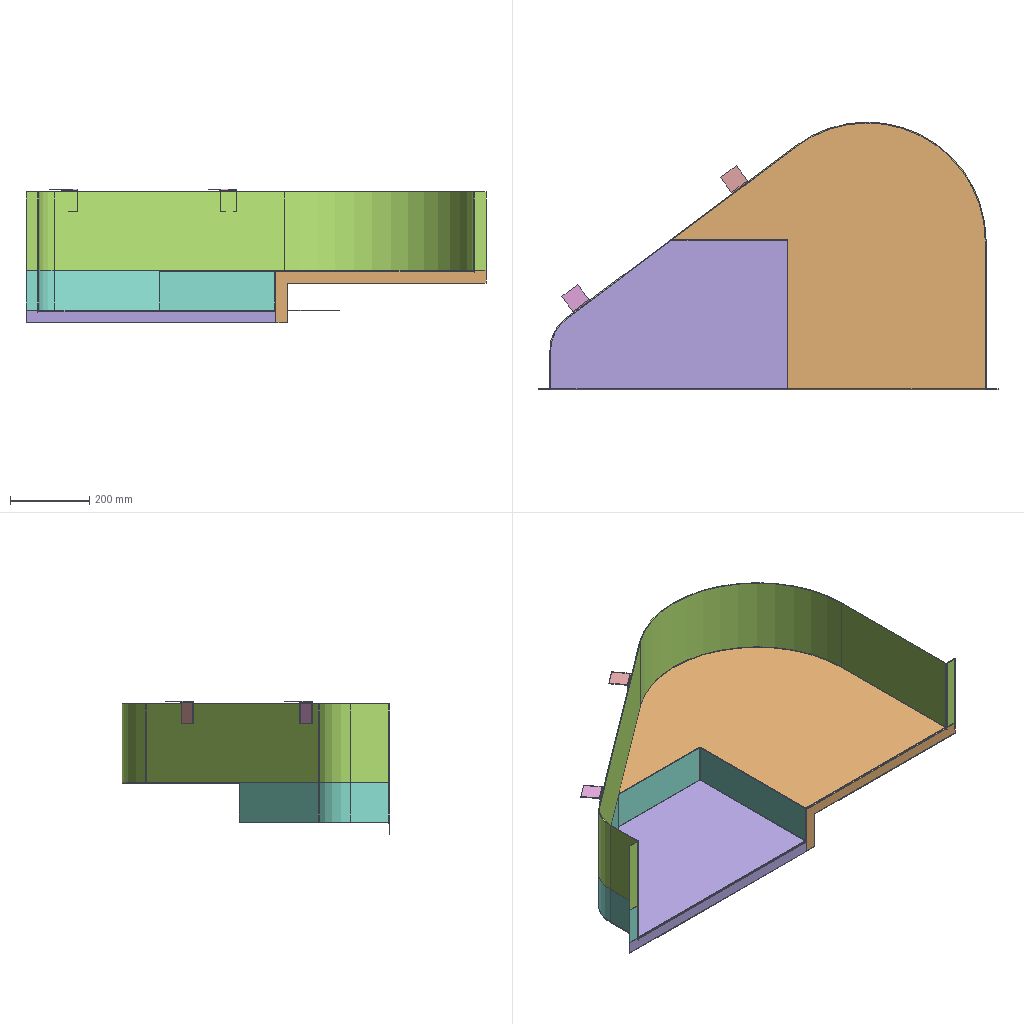Assembly | SolidWorks | 8 different items | 8 placed | box 1160 x 675 x 337 mm
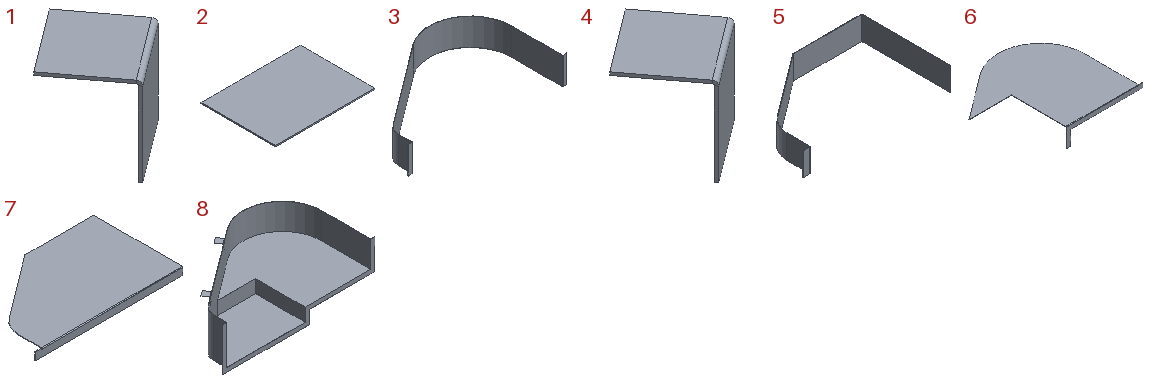Parts list (item | quantity | size | volume | features):
1 | x1 | 70 x 70 x 57 mm | 10414 mm3 | features ICE 5, Split 2, DeleteBody 1, Extrusion 1, FlatPattern 1, SheetMetal 1, Shell 1, SolidToSheetMetal 1
2 | x1 | 160 x 120 x 2 mm | 38400 mm3 | features ICE 5, SheetMetal 2, SolidToSheetMetal 2, DeleteBody 1, Extrusion 1, FlatPattern 1, Shell 1
3 | x1 | 1160 x 675 x 198 mm | 796815 mm3 | features ICE 5, SheetMetal 3, SolidToSheetMetal 3, DeleteBody 1, Extrusion 1, FlatPattern 1, Shell 1, Split 1
4 | x1 | 70 x 70 x 57 mm | 10414 mm3 | features ICE 5, DeleteBody 1, Extrusion 1, FlatPattern 1, SheetMetal 1, Shell 1, SolidToSheetMetal 1
5 | x1 | 630 x 380 x 100 mm | 244808 mm3 | features ICE 5, DeleteBody 4, Split 4, Extrusion 1, FlatPattern 1, SheetMetal 1, Shell 1, SolidToSheetMetal 1
6 | x1 | 823.333 x 675 x 132 mm | 728370 mm3 | features ICE 5, DeleteBody 3, Split 3, CombineBodies 1, Extrusion 1, FlatPattern 1, SheetMetal 1, Shell 1, SolidToSheetMetal 1
7 | x1 | 630 x 380 x 32 mm | 421618 mm3 | features ICE 5, Split 4, DeleteBody 3, Extrusion 1, FlatPattern 1, SheetMetal 1, Shell 1, SolidToSheetMetal 1
8 | x1 | 1160 x 675 x 337 mm | 2407556 mm3 | features ICE 5, Extrusion 1, Shell 1
Mates (type | each side: item.copy, entity, surface, feature):
Coincident | 1.1 face plane Convert entity 1 | 3.1 face plane Convert entity 3
DistanceDim | 3.1 edge | 1.1 edge
DistanceDim | 1.1 face plane Convert entity 1 | 3.1 face plane Convert entity 3
DistanceDim | 1.1 face plane Convert entity 1 | 4.1 face plane Convert entity 1
Coincident | 3.1 face plane Convert entity 3 | 4.1 face plane Convert entity 1
Coincident | 1.1 edge | 4.1 edge
Coincident | 3.1 edge | 6.1 edge
Coincident | 3.1 face plane Convert entity 3 | 6.1 face plane Convert entity 1
Coincident | 3.1 edge | 5.1 edge
Coincident | 3.1 face plane Convert entity 3 | 5.1 face plane Convert entity 1
Coincident | 5.1 edge | 7.1 face plane Convert entity 1
Coincident | 6.1 edge | 7.1 edge
Coincident | 6.1 face plane Convert entity 1 | 7.1 face plane Convert entity 1
Coincident | 2.1 face plane Convert entity 2 | 7.1 face plane Convert entity 1
Coincident | 2.1 edge | 5.1 face plane Convert entity 1
Coincident | 2.1 face plane Convert entity 2 | 5.1 face plane Convert entity 1